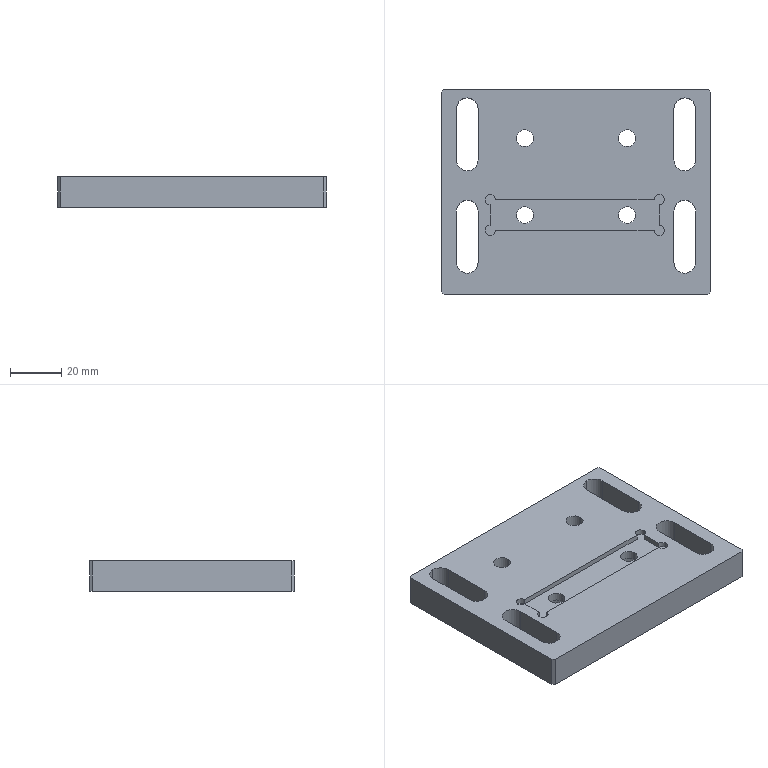Part | 1 solid | 59 faces | box 105 x 80 x 12 mm | volume 85078 mm3 | cylinder 32 | plane 27 | commonest cylinder face diameters 8.5 x10 6.6 x8 11 x8 4 x6